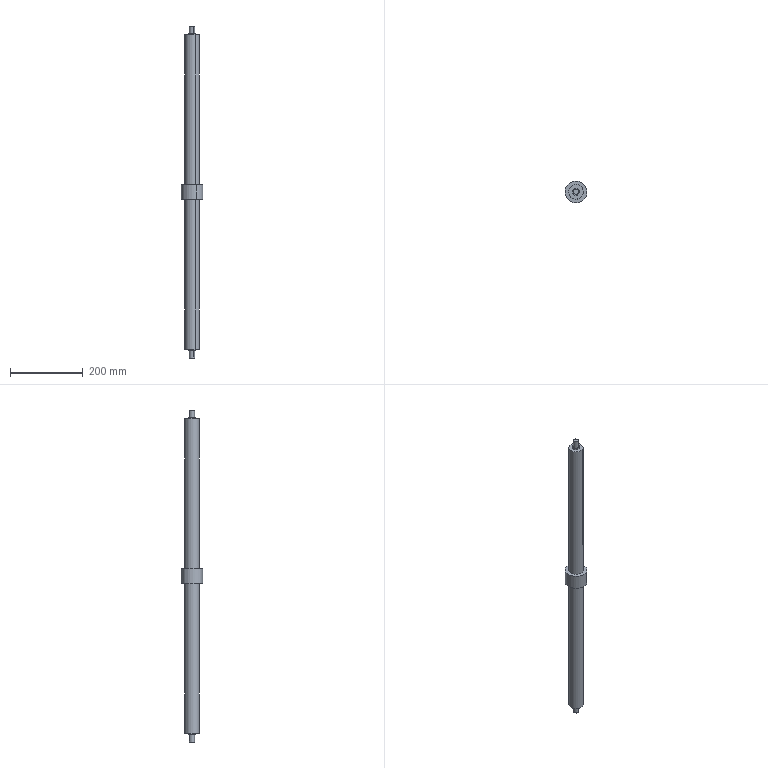Part | SolidWorks | features BaseBody 1 | 1 solid | 34 faces | box 60 x 60 x 912 mm | volume 1156729 mm3 | plane 24 | cylinder 10 | commonest cylinder face diameters 14 x4 40 x4 60 x2
STEP:
#1=CARTESIAN_POINT('',(-440.034,50.813,456.));
#2=VERTEX_POINT('',#1);
#3=CARTESIAN_POINT('',(-446.031,63.464,456.));
#4=VERTEX_POINT('',#3);
#5=CARTESIAN_POINT('',(-443.032,57.138,456.));
#6=DIRECTION('',(0.,0.,1.));
#7=DIRECTION('',(0.4284,-0.9036,0.));
#8=AXIS2_PLACEMENT_3D('',#5,#6,#7);
#9=CIRCLE('',#8,7.);
#10=EDGE_CURVE('',#2,#4,#9,.T.);
#11=ORIENTED_EDGE('',*,*,#10,.F.);
#12=CARTESIAN_POINT('',(-440.034,50.813,435.));
#13=VERTEX_POINT('',#12);
#14=CARTESIAN_POINT('',(-440.034,50.813,456.));
#15=DIRECTION('',(0.,0.,-1.));
#16=VECTOR('',#15,1000.);
#17=LINE('',#14,#16);
#18=EDGE_CURVE('',#2,#13,#17,.T.);
#19=ORIENTED_EDGE('',*,*,#18,.T.);
#20=CARTESIAN_POINT('',(-446.031,63.464,435.));
#21=VERTEX_POINT('',#20);
#22=CARTESIAN_POINT('',(-443.032,57.138,435.));
#23=DIRECTION('',(0.,0.,1.));
#24=DIRECTION('',(0.4284,-0.9036,0.));
#25=AXIS2_PLACEMENT_3D('',#22,#23,#24);
#26=CIRCLE('',#25,7.);
#27=EDGE_CURVE('',#13,#21,#26,.T.);
#28=ORIENTED_EDGE('',*,*,#27,.T.);
#29=CARTESIAN_POINT('',(-446.031,63.464,456.));
#30=DIRECTION('',(0.,0.,-1.));
#31=VECTOR('',#30,1000.);
#32=LINE('',#29,#31);
#33=EDGE_CURVE('',#4,#21,#32,.T.);
#34=ORIENTED_EDGE('',*,*,#33,.F.);
#35=EDGE_LOOP('',(#11,#19,#28,#34));
#36=FACE_OUTER_BOUND('',#35,.T.);
#37=CARTESIAN_POINT('',(-443.032,57.138,456.));
#38=DIRECTION('',(0.,0.,-1.));
#39=DIRECTION('',(-0.4284,0.9036,0.));
#40=AXIS2_PLACEMENT_3D('',#37,#38,#39);
#41=CYLINDRICAL_SURFACE('',#40,7.);
#42=ADVANCED_FACE('',(#36),#41,.T.);
#43=CARTESIAN_POINT('',(-446.031,63.464,-456.));
#44=VERTEX_POINT('',#43);
#45=CARTESIAN_POINT('',(-440.034,50.813,-456.));
#46=VERTEX_POINT('',#45);
#47=CARTESIAN_POINT('',(-443.032,57.138,-456.));
#48=DIRECTION('',(0.,0.,-1.));
#49=DIRECTION('',(-0.4284,0.9036,0.));
#50=AXIS2_PLACEMENT_3D('',#47,#48,#49);
#51=CIRCLE('',#50,7.);
#52=EDGE_CURVE('',#44,#46,#51,.T.);
#53=ORIENTED_EDGE('',*,*,#52,.F.);
#54=CARTESIAN_POINT('',(-446.031,63.464,-435.));
#55=VERTEX_POINT('',#54);
#56=CARTESIAN_POINT('',(-446.031,63.464,-456.));
#57=DIRECTION('',(0.,0.,1.));
#58=VECTOR('',#57,1000.);
#59=LINE('',#56,#58);
#60=EDGE_CURVE('',#44,#55,#59,.T.);
#61=ORIENTED_EDGE('',*,*,#60,.T.);
#62=CARTESIAN_POINT('',(-440.034,50.813,-435.));
#63=VERTEX_POINT('',#62);
#64=CARTESIAN_POINT('',(-443.032,57.138,-435.));
#65=DIRECTION('',(0.,0.,-1.));
#66=DIRECTION('',(-0.4284,0.9036,0.));
#67=AXIS2_PLACEMENT_3D('',#64,#65,#66);
#68=CIRCLE('',#67,7.);
#69=EDGE_CURVE('',#55,#63,#68,.T.);
#70=ORIENTED_EDGE('',*,*,#69,.T.);
#71=CARTESIAN_POINT('',(-440.034,50.813,-456.));
#72=DIRECTION('',(0.,0.,1.));
#73=VECTOR('',#72,1000.);
#74=LINE('',#71,#73);
#75=EDGE_CURVE('',#46,#63,#74,.T.);
#76=ORIENTED_EDGE('',*,*,#75,.F.);
#77=EDGE_LOOP('',(#53,#61,#70,#76));
#78=FACE_OUTER_BOUND('',#77,.T.);
#79=CARTESIAN_POINT('',(-443.032,57.138,-456.));
#80=DIRECTION('',(0.,0.,1.));
#81=DIRECTION('',(0.4284,-0.9036,0.));
#82=AXIS2_PLACEMENT_3D('',#79,#80,#81);
#83=CYLINDRICAL_SURFACE('',#82,7.);
#84=ADVANCED_FACE('',(#78),#83,.T.);
#85=CARTESIAN_POINT('',(-430.181,30.03,20.));
#86=VERTEX_POINT('',#85);
#87=CARTESIAN_POINT('',(-455.884,84.246,20.));
#88=VERTEX_POINT('',#87);
#89=CARTESIAN_POINT('',(-443.032,57.138,20.));
#90=DIRECTION('',(0.,0.,1.));
#91=DIRECTION('',(0.4284,-0.9036,0.));
#92=AXIS2_PLACEMENT_3D('',#89,#90,#91);
#93=CIRCLE('',#92,30.);
#94=EDGE_CURVE('',#86,#88,#93,.T.);
#95=ORIENTED_EDGE('',*,*,#94,.F.);
#96=CARTESIAN_POINT('',(-430.181,30.03,-20.));
#97=VERTEX_POINT('',#96);
#98=CARTESIAN_POINT('',(-430.181,30.03,20.));
#99=DIRECTION('',(0.,0.,-1.));
#100=VECTOR('',#99,1000.);
#101=LINE('',#98,#100);
#102=EDGE_CURVE('',#86,#97,#101,.T.);
#103=ORIENTED_EDGE('',*,*,#102,.T.);
#104=CARTESIAN_POINT('',(-455.884,84.246,-20.));
#105=VERTEX_POINT('',#104);
#106=CARTESIAN_POINT('',(-443.032,57.138,-20.));
#107=DIRECTION('',(0.,0.,1.));
#108=DIRECTION('',(0.4284,-0.9036,0.));
#109=AXIS2_PLACEMENT_3D('',#106,#107,#108);
#110=CIRCLE('',#109,30.);
#111=EDGE_CURVE('',#97,#105,#110,.T.);
#112=ORIENTED_EDGE('',*,*,#111,.T.);
#113=CARTESIAN_POINT('',(-455.884,84.246,20.));
#114=DIRECTION('',(0.,0.,-1.));
#115=VECTOR('',#114,1000.);
#116=LINE('',#113,#115);
#117=EDGE_CURVE('',#88,#105,#116,.T.);
#118=ORIENTED_EDGE('',*,*,#117,.F.);
#119=EDGE_LOOP('',(#95,#103,#112,#118));
#120=FACE_OUTER_BOUND('',#119,.T.);
#121=CARTESIAN_POINT('',(-443.032,57.138,20.));
#122=DIRECTION('',(0.,0.,-1.));
#123=DIRECTION('',(-0.4284,0.9036,0.));
#124=AXIS2_PLACEMENT_3D('',#121,#122,#123);
#125=CYLINDRICAL_SURFACE('',#124,30.);
#126=ADVANCED_FACE('',(#120),#125,.T.);
#127=CARTESIAN_POINT('',(-434.465,39.066,-20.));
#128=VERTEX_POINT('',#127);
#129=CARTESIAN_POINT('',(-451.6,75.21,-20.));
#130=VERTEX_POINT('',#129);
#131=CARTESIAN_POINT('',(-443.032,57.138,-20.));
#132=DIRECTION('',(0.,0.,1.));
#133=DIRECTION('',(0.4284,-0.9036,0.));
#134=AXIS2_PLACEMENT_3D('',#131,#132,#133);
#135=CIRCLE('',#134,20.);
#136=EDGE_CURVE('',#128,#130,#135,.T.);
#137=ORIENTED_EDGE('',*,*,#136,.F.);
#138=CARTESIAN_POINT('',(-434.465,39.066,-432.));
#139=VERTEX_POINT('',#138);
#140=CARTESIAN_POINT('',(-434.465,39.066,445.));
#141=DIRECTION('',(0.,0.,-1.));
#142=VECTOR('',#141,1000.);
#143=LINE('',#140,#142);
#144=EDGE_CURVE('',#128,#139,#143,.T.);
#145=ORIENTED_EDGE('',*,*,#144,.T.);
#146=CARTESIAN_POINT('',(-451.6,75.21,-432.));
#147=VERTEX_POINT('',#146);
#148=CARTESIAN_POINT('',(-443.032,57.138,-432.));
#149=DIRECTION('',(0.,0.,-1.));
#150=DIRECTION('',(-0.4284,0.9036,0.));
#151=AXIS2_PLACEMENT_3D('',#148,#149,#150);
#152=CIRCLE('',#151,20.);
#153=EDGE_CURVE('',#147,#139,#152,.T.);
#154=ORIENTED_EDGE('',*,*,#153,.F.);
#155=CARTESIAN_POINT('',(-451.6,75.21,445.));
#156=DIRECTION('',(0.,0.,-1.));
#157=VECTOR('',#156,1000.);
#158=LINE('',#155,#157);
#159=EDGE_CURVE('',#130,#147,#158,.T.);
#160=ORIENTED_EDGE('',*,*,#159,.F.);
#161=EDGE_LOOP('',(#137,#145,#154,#160));
#162=FACE_OUTER_BOUND('',#161,.T.);
#163=CARTESIAN_POINT('',(-443.032,57.138,445.));
#164=DIRECTION('',(0.,0.,-1.));
#165=DIRECTION('',(-0.4284,0.9036,0.));
#166=AXIS2_PLACEMENT_3D('',#163,#164,#165);
#167=CYLINDRICAL_SURFACE('',#166,20.);
#168=ADVANCED_FACE('',(#162),#167,.T.);
#169=CARTESIAN_POINT('',(-434.465,39.066,432.));
#170=VERTEX_POINT('',#169);
#171=CARTESIAN_POINT('',(-451.6,75.21,432.));
#172=VERTEX_POINT('',#171);
#173=CARTESIAN_POINT('',(-443.032,57.138,432.));
#174=DIRECTION('',(0.,0.,1.));
#175=DIRECTION('',(0.4284,-0.9036,0.));
#176=AXIS2_PLACEMENT_3D('',#173,#174,#175);
#177=CIRCLE('',#176,20.);
#178=EDGE_CURVE('',#170,#172,#177,.T.);
#179=ORIENTED_EDGE('',*,*,#178,.F.);
#180=CARTESIAN_POINT('',(-434.465,39.066,20.));
#181=VERTEX_POINT('',#180);
#182=CARTESIAN_POINT('',(-434.465,39.066,445.));
#183=DIRECTION('',(0.,0.,-1.));
#184=VECTOR('',#183,1000.);
#185=LINE('',#182,#184);
#186=EDGE_CURVE('',#170,#181,#185,.T.);
#187=ORIENTED_EDGE('',*,*,#186,.T.);
#188=CARTESIAN_POINT('',(-451.6,75.21,20.));
#189=VERTEX_POINT('',#188);
#190=CARTESIAN_POINT('',(-443.032,57.138,20.));
#191=DIRECTION('',(0.,0.,1.));
#192=DIRECTION('',(0.4284,-0.9036,0.));
#193=AXIS2_PLACEMENT_3D('',#190,#191,#192);
#194=CIRCLE('',#193,20.);
#195=EDGE_CURVE('',#181,#189,#194,.T.);
#196=ORIENTED_EDGE('',*,*,#195,.T.);
#197=CARTESIAN_POINT('',(-451.6,75.21,445.));
#198=DIRECTION('',(0.,0.,-1.));
#199=VECTOR('',#198,1000.);
#200=LINE('',#197,#199);
#201=EDGE_CURVE('',#172,#189,#200,.T.);
#202=ORIENTED_EDGE('',*,*,#201,.F.);
#203=EDGE_LOOP('',(#179,#187,#196,#202));
#204=FACE_OUTER_BOUND('',#203,.T.);
#205=CARTESIAN_POINT('',(-443.032,57.138,445.));
#206=DIRECTION('',(0.,0.,-1.));
#207=DIRECTION('',(-0.4284,0.9036,0.));
#208=AXIS2_PLACEMENT_3D('',#205,#206,#207);
#209=CYLINDRICAL_SURFACE('',#208,20.);
#210=ADVANCED_FACE('',(#204),#209,.T.);
#211=ORIENTED_EDGE('',*,*,#186,.F.);
#212=CARTESIAN_POINT('',(-443.032,57.138,432.));
#213=DIRECTION('',(0.,0.,1.));
#214=DIRECTION('',(0.4284,-0.9036,0.));
#215=AXIS2_PLACEMENT_3D('',#212,#213,#214);
#216=CIRCLE('',#215,20.);
#217=EDGE_CURVE('',#172,#170,#216,.T.);
#218=ORIENTED_EDGE('',*,*,#217,.F.);
#219=ORIENTED_EDGE('',*,*,#201,.T.);
#220=CARTESIAN_POINT('',(-443.032,57.138,20.));
#221=DIRECTION('',(0.,0.,1.));
#222=DIRECTION('',(0.4284,-0.9036,0.));
#223=AXIS2_PLACEMENT_3D('',#220,#221,#222);
#224=CIRCLE('',#223,20.);
#225=EDGE_CURVE('',#189,#181,#224,.T.);
#226=ORIENTED_EDGE('',*,*,#225,.T.);
#227=EDGE_LOOP('',(#211,#218,#219,#226));
#228=FACE_OUTER_BOUND('',#227,.T.);
#229=CARTESIAN_POINT('',(-443.032,57.138,445.));
#230=DIRECTION('',(0.,0.,-1.));
#231=DIRECTION('',(-0.4284,0.9036,0.));
#232=AXIS2_PLACEMENT_3D('',#229,#230,#231);
#233=CYLINDRICAL_SURFACE('',#232,20.);
#234=ADVANCED_FACE('',(#228),#233,.T.);
#235=ORIENTED_EDGE('',*,*,#144,.F.);
#236=CARTESIAN_POINT('',(-443.032,57.138,-20.));
#237=DIRECTION('',(0.,0.,1.));
#238=DIRECTION('',(0.4284,-0.9036,0.));
#239=AXIS2_PLACEMENT_3D('',#236,#237,#238);
#240=CIRCLE('',#239,20.);
#241=EDGE_CURVE('',#130,#128,#240,.T.);
#242=ORIENTED_EDGE('',*,*,#241,.F.);
#243=ORIENTED_EDGE('',*,*,#159,.T.);
#244=CARTESIAN_POINT('',(-443.032,57.138,-432.));
#245=DIRECTION('',(0.,0.,-1.));
#246=DIRECTION('',(-0.4284,0.9036,0.));
#247=AXIS2_PLACEMENT_3D('',#244,#245,#246);
#248=CIRCLE('',#247,20.);
#249=EDGE_CURVE('',#139,#147,#248,.T.);
#250=ORIENTED_EDGE('',*,*,#249,.F.);
#251=EDGE_LOOP('',(#235,#242,#243,#250));
#252=FACE_OUTER_BOUND('',#251,.T.);
#253=CARTESIAN_POINT('',(-443.032,57.138,445.));
#254=DIRECTION('',(0.,0.,-1.));
#255=DIRECTION('',(-0.4284,0.9036,0.));
#256=AXIS2_PLACEMENT_3D('',#253,#254,#255);
#257=CYLINDRICAL_SURFACE('',#256,20.);
#258=ADVANCED_FACE('',(#252),#257,.T.);
#259=CARTESIAN_POINT('',(-443.032,57.138,20.));
#260=DIRECTION('',(0.,0.,1.));
#261=DIRECTION('',(0.4284,-0.9036,0.));
#262=AXIS2_PLACEMENT_3D('',#259,#260,#261);
#263=CIRCLE('',#262,30.);
#264=EDGE_CURVE('',#88,#86,#263,.T.);
#265=ORIENTED_EDGE('',*,*,#264,.T.);
#266=ORIENTED_EDGE('',*,*,#94,.T.);
#267=EDGE_LOOP('',(#265,#266));
#268=FACE_OUTER_BOUND('',#267,.T.);
#269=ORIENTED_EDGE('',*,*,#225,.F.);
#270=ORIENTED_EDGE('',*,*,#195,.F.);
#271=EDGE_LOOP('',(#269,#270));
#272=FACE_BOUND('',#271,.T.);
#273=CARTESIAN_POINT('',(-443.032,57.138,20.));
#274=DIRECTION('',(0.,0.,1.));
#275=DIRECTION('',(0.4284,-0.9036,0.));
#276=AXIS2_PLACEMENT_3D('',#273,#274,#275);
#277=PLANE('',#276);
#278=ADVANCED_FACE('',(#268,#272),#277,.T.);
#279=CARTESIAN_POINT('',(-443.032,57.138,-20.));
#280=DIRECTION('',(0.,0.,1.));
#281=DIRECTION('',(0.4284,-0.9036,0.));
#282=AXIS2_PLACEMENT_3D('',#279,#280,#281);
#283=CIRCLE('',#282,30.);
#284=EDGE_CURVE('',#105,#97,#283,.T.);
#285=ORIENTED_EDGE('',*,*,#284,.F.);
#286=ORIENTED_EDGE('',*,*,#111,.F.);
#287=EDGE_LOOP('',(#285,#286));
#288=FACE_OUTER_BOUND('',#287,.T.);
#289=ORIENTED_EDGE('',*,*,#241,.T.);
#290=ORIENTED_EDGE('',*,*,#136,.T.);
#291=EDGE_LOOP('',(#289,#290));
#292=FACE_BOUND('',#291,.T.);
#293=CARTESIAN_POINT('',(-443.032,57.138,-20.));
#294=DIRECTION('',(0.,0.,1.));
#295=DIRECTION('',(0.4284,-0.9036,0.));
#296=AXIS2_PLACEMENT_3D('',#293,#294,#295);
#297=PLANE('',#296);
#298=ADVANCED_FACE('',(#288,#292),#297,.F.);
#299=ORIENTED_EDGE('',*,*,#102,.F.);
#300=ORIENTED_EDGE('',*,*,#264,.F.);
#301=ORIENTED_EDGE('',*,*,#117,.T.);
#302=ORIENTED_EDGE('',*,*,#284,.T.);
#303=EDGE_LOOP('',(#299,#300,#301,#302));
#304=FACE_OUTER_BOUND('',#303,.T.);
#305=CARTESIAN_POINT('',(-443.032,57.138,20.));
#306=DIRECTION('',(0.,0.,-1.));
#307=DIRECTION('',(-0.4284,0.9036,0.));
#308=AXIS2_PLACEMENT_3D('',#305,#306,#307);
#309=CYLINDRICAL_SURFACE('',#308,30.);
#310=ADVANCED_FACE('',(#304),#309,.T.);
#311=ORIENTED_EDGE('',*,*,#153,.T.);
#312=ORIENTED_EDGE('',*,*,#249,.T.);
#313=EDGE_LOOP('',(#311,#312));
#314=FACE_OUTER_BOUND('',#313,.T.);
#315=CARTESIAN_POINT('',(-447.316,66.174,-432.));
#316=VERTEX_POINT('',#315);
#317=CARTESIAN_POINT('',(-439.672,66.557,-432.));
#318=VERTEX_POINT('',#317);
#319=CARTESIAN_POINT('',(-439.672,66.557,-432.));
#320=DIRECTION('',(0.9987,0.04998,0.));
#321=VECTOR('',#320,1000.);
#322=LINE('',#319,#321);
#323=EDGE_CURVE('',#316,#318,#322,.T.);
#324=ORIENTED_EDGE('',*,*,#323,.F.);
#325=CARTESIAN_POINT('',(-452.451,60.499,-432.));
#326=VERTEX_POINT('',#325);
#327=CARTESIAN_POINT('',(-452.451,60.499,-432.));
#328=DIRECTION('',(0.6709,0.7416,0.));
#329=VECTOR('',#328,1000.);
#330=LINE('',#327,#329);
#331=EDGE_CURVE('',#326,#316,#330,.T.);
#332=ORIENTED_EDGE('',*,*,#331,.F.);
#333=CARTESIAN_POINT('',(-452.068,52.855,-432.));
#334=VERTEX_POINT('',#333);
#335=CARTESIAN_POINT('',(-452.068,52.855,-432.));
#336=DIRECTION('',(-0.04998,0.9987,0.));
#337=VECTOR('',#336,1000.);
#338=LINE('',#335,#337);
#339=EDGE_CURVE('',#334,#326,#338,.T.);
#340=ORIENTED_EDGE('',*,*,#339,.F.);
#341=CARTESIAN_POINT('',(-446.393,47.72,-432.));
#342=VERTEX_POINT('',#341);
#343=CARTESIAN_POINT('',(-452.068,52.855,-432.));
#344=DIRECTION('',(-0.7416,0.6709,0.));
#345=VECTOR('',#344,1000.);
#346=LINE('',#343,#345);
#347=EDGE_CURVE('',#342,#334,#346,.T.);
#348=ORIENTED_EDGE('',*,*,#347,.F.);
#349=CARTESIAN_POINT('',(-438.748,48.102,-432.));
#350=VERTEX_POINT('',#349);
#351=CARTESIAN_POINT('',(-446.393,47.72,-432.));
#352=DIRECTION('',(-0.9987,-0.04998,0.));
#353=VECTOR('',#352,1000.);
#354=LINE('',#351,#353);
#355=EDGE_CURVE('',#350,#342,#354,.T.);
#356=ORIENTED_EDGE('',*,*,#355,.F.);
#357=CARTESIAN_POINT('',(-433.614,53.778,-432.));
#358=VERTEX_POINT('',#357);
#359=CARTESIAN_POINT('',(-433.614,53.778,-432.));
#360=DIRECTION('',(-0.6709,-0.7416,0.));
#361=VECTOR('',#360,1000.);
#362=LINE('',#359,#361);
#363=EDGE_CURVE('',#358,#350,#362,.T.);
#364=ORIENTED_EDGE('',*,*,#363,.F.);
#365=CARTESIAN_POINT('',(-433.996,61.422,-432.));
#366=VERTEX_POINT('',#365);
#367=CARTESIAN_POINT('',(-433.996,61.422,-432.));
#368=DIRECTION('',(0.04998,-0.9987,0.));
#369=VECTOR('',#368,1000.);
#370=LINE('',#367,#369);
#371=EDGE_CURVE('',#366,#358,#370,.T.);
#372=ORIENTED_EDGE('',*,*,#371,.F.);
#373=CARTESIAN_POINT('',(-433.996,61.422,-432.));
#374=DIRECTION('',(0.7416,-0.6709,0.));
#375=VECTOR('',#374,1000.);
#376=LINE('',#373,#375);
#377=EDGE_CURVE('',#318,#366,#376,.T.);
#378=ORIENTED_EDGE('',*,*,#377,.F.);
#379=EDGE_LOOP('',(#324,#332,#340,#348,#356,#364,#372,#378));
#380=FACE_BOUND('',#379,.T.);
#381=CARTESIAN_POINT('',(-443.032,57.138,-432.));
#382=DIRECTION('',(0.,0.,-1.));
#383=DIRECTION('',(-0.4284,0.9036,0.));
#384=AXIS2_PLACEMENT_3D('',#381,#382,#383);
#385=PLANE('',#384);
#386=ADVANCED_FACE('',(#314,#380),#385,.T.);
#387=CARTESIAN_POINT('',(-439.672,66.557,-435.));
#388=VERTEX_POINT('',#387);
#389=CARTESIAN_POINT('',(-433.996,61.422,-435.));
#390=VERTEX_POINT('',#389);
#391=CARTESIAN_POINT('',(-433.996,61.422,-435.));
#392=DIRECTION('',(0.7416,-0.6709,0.));
#393=VECTOR('',#392,1000.);
#394=LINE('',#391,#393);
#395=EDGE_CURVE('',#388,#390,#394,.T.);
#396=ORIENTED_EDGE('',*,*,#395,.F.);
#397=CARTESIAN_POINT('',(-439.672,66.557,-432.));
#398=DIRECTION('',(0.,0.,-1.));
#399=VECTOR('',#398,1000.);
#400=LINE('',#397,#399);
#401=EDGE_CURVE('',#318,#388,#400,.T.);
#402=ORIENTED_EDGE('',*,*,#401,.F.);
#403=ORIENTED_EDGE('',*,*,#377,.T.);
#404=CARTESIAN_POINT('',(-433.996,61.422,-432.));
#405=DIRECTION('',(0.,0.,-1.));
#406=VECTOR('',#405,1000.);
#407=LINE('',#404,#406);
#408=EDGE_CURVE('',#366,#390,#407,.T.);
#409=ORIENTED_EDGE('',*,*,#408,.T.);
#410=EDGE_LOOP('',(#396,#402,#403,#409));
#411=FACE_OUTER_BOUND('',#410,.T.);
#412=CARTESIAN_POINT('',(-433.996,61.422,-432.));
#413=DIRECTION('',(0.6709,0.7416,0.));
#414=DIRECTION('',(-0.7416,0.6709,0.));
#415=AXIS2_PLACEMENT_3D('',#412,#413,#414);
#416=PLANE('',#415);
#417=ADVANCED_FACE('',(#411),#416,.T.);
#418=CARTESIAN_POINT('',(-447.316,66.174,-435.));
#419=VERTEX_POINT('',#418);
#420=CARTESIAN_POINT('',(-439.672,66.557,-435.));
#421=DIRECTION('',(0.9987,0.04998,0.));
#422=VECTOR('',#421,1000.);
#423=LINE('',#420,#422);
#424=EDGE_CURVE('',#419,#388,#423,.T.);
#425=ORIENTED_EDGE('',*,*,#424,.F.);
#426=CARTESIAN_POINT('',(-447.316,66.174,-432.));
#427=DIRECTION('',(0.,0.,-1.));
#428=VECTOR('',#427,1000.);
#429=LINE('',#426,#428);
#430=EDGE_CURVE('',#316,#419,#429,.T.);
#431=ORIENTED_EDGE('',*,*,#430,.F.);
#432=ORIENTED_EDGE('',*,*,#323,.T.);
#433=ORIENTED_EDGE('',*,*,#401,.T.);
#434=EDGE_LOOP('',(#425,#431,#432,#433));
#435=FACE_OUTER_BOUND('',#434,.T.);
#436=CARTESIAN_POINT('',(-439.672,66.557,-432.));
#437=DIRECTION('',(-0.04998,0.9987,0.));
#438=DIRECTION('',(-0.9987,-0.04998,0.));
#439=AXIS2_PLACEMENT_3D('',#436,#437,#438);
#440=PLANE('',#439);
#441=ADVANCED_FACE('',(#435),#440,.T.);
#442=CARTESIAN_POINT('',(-452.451,60.499,-435.));
#443=VERTEX_POINT('',#442);
#444=CARTESIAN_POINT('',(-452.451,60.499,-435.));
#445=DIRECTION('',(0.6709,0.7416,0.));
#446=VECTOR('',#445,1000.);
#447=LINE('',#444,#446);
#448=EDGE_CURVE('',#443,#419,#447,.T.);
#449=ORIENTED_EDGE('',*,*,#448,.F.);
#450=CARTESIAN_POINT('',(-452.451,60.499,-432.));
#451=DIRECTION('',(0.,0.,-1.));
#452=VECTOR('',#451,1000.);
#453=LINE('',#450,#452);
#454=EDGE_CURVE('',#326,#443,#453,.T.);
#455=ORIENTED_EDGE('',*,*,#454,.F.);
#456=ORIENTED_EDGE('',*,*,#331,.T.);
#457=ORIENTED_EDGE('',*,*,#430,.T.);
#458=EDGE_LOOP('',(#449,#455,#456,#457));
#459=FACE_OUTER_BOUND('',#458,.T.);
#460=CARTESIAN_POINT('',(-452.451,60.499,-432.));
#461=DIRECTION('',(-0.7416,0.6709,0.));
#462=DIRECTION('',(-0.6709,-0.7416,0.));
#463=AXIS2_PLACEMENT_3D('',#460,#461,#462);
#464=PLANE('',#463);
#465=ADVANCED_FACE('',(#459),#464,.T.);
#466=CARTESIAN_POINT('',(-452.068,52.855,-435.));
#467=VERTEX_POINT('',#466);
#468=CARTESIAN_POINT('',(-452.068,52.855,-435.));
#469=DIRECTION('',(-0.04998,0.9987,0.));
#470=VECTOR('',#469,1000.);
#471=LINE('',#468,#470);
#472=EDGE_CURVE('',#467,#443,#471,.T.);
#473=ORIENTED_EDGE('',*,*,#472,.F.);
#474=CARTESIAN_POINT('',(-452.068,52.855,-432.));
#475=DIRECTION('',(0.,0.,-1.));
#476=VECTOR('',#475,1000.);
#477=LINE('',#474,#476);
#478=EDGE_CURVE('',#334,#467,#477,.T.);
#479=ORIENTED_EDGE('',*,*,#478,.F.);
#480=ORIENTED_EDGE('',*,*,#339,.T.);
#481=ORIENTED_EDGE('',*,*,#454,.T.);
#482=EDGE_LOOP('',(#473,#479,#480,#481));
#483=FACE_OUTER_BOUND('',#482,.T.);
#484=CARTESIAN_POINT('',(-452.068,52.855,-432.));
#485=DIRECTION('',(-0.9987,-0.04998,0.));
#486=DIRECTION('',(0.04998,-0.9987,0.));
#487=AXIS2_PLACEMENT_3D('',#484,#485,#486);
#488=PLANE('',#487);
#489=ADVANCED_FACE('',(#483),#488,.T.);
#490=CARTESIAN_POINT('',(-446.393,47.72,-435.));
#491=VERTEX_POINT('',#490);
#492=CARTESIAN_POINT('',(-452.068,52.855,-435.));
#493=DIRECTION('',(-0.7416,0.6709,0.));
#494=VECTOR('',#493,1000.);
#495=LINE('',#492,#494);
#496=EDGE_CURVE('',#491,#467,#495,.T.);
#497=ORIENTED_EDGE('',*,*,#496,.F.);
#498=CARTESIAN_POINT('',(-446.393,47.72,-432.));
#499=DIRECTION('',(0.,0.,-1.));
#500=VECTOR('',#499,1000.);
#501=LINE('',#498,#500);
#502=EDGE_CURVE('',#342,#491,#501,.T.);
#503=ORIENTED_EDGE('',*,*,#502,.F.);
#504=ORIENTED_EDGE('',*,*,#347,.T.);
#505=ORIENTED_EDGE('',*,*,#478,.T.);
#506=EDGE_LOOP('',(#497,#503,#504,#505));
#507=FACE_OUTER_BOUND('',#506,.T.);
#508=CARTESIAN_POINT('',(-452.068,52.855,-432.));
#509=DIRECTION('',(-0.6709,-0.7416,0.));
#510=DIRECTION('',(0.7416,-0.6709,0.));
#511=AXIS2_PLACEMENT_3D('',#508,#509,#510);
#512=PLANE('',#511);
#513=ADVANCED_FACE('',(#507),#512,.T.);
#514=CARTESIAN_POINT('',(-438.748,48.102,-435.));
#515=VERTEX_POINT('',#514);
#516=CARTESIAN_POINT('',(-446.393,47.72,-435.));
#517=DIRECTION('',(-0.9987,-0.04998,0.));
#518=VECTOR('',#517,1000.);
#519=LINE('',#516,#518);
#520=EDGE_CURVE('',#515,#491,#519,.T.);
#521=ORIENTED_EDGE('',*,*,#520,.F.);
#522=CARTESIAN_POINT('',(-438.748,48.102,-432.));
#523=DIRECTION('',(0.,0.,-1.));
#524=VECTOR('',#523,1000.);
#525=LINE('',#522,#524);
#526=EDGE_CURVE('',#350,#515,#525,.T.);
#527=ORIENTED_EDGE('',*,*,#526,.F.);
#528=ORIENTED_EDGE('',*,*,#355,.T.);
#529=ORIENTED_EDGE('',*,*,#502,.T.);
#530=EDGE_LOOP('',(#521,#527,#528,#529));
#531=FACE_OUTER_BOUND('',#530,.T.);
#532=CARTESIAN_POINT('',(-446.393,47.72,-432.));
#533=DIRECTION('',(0.04998,-0.9987,0.));
#534=DIRECTION('',(0.9987,0.04998,0.));
#535=AXIS2_PLACEMENT_3D('',#532,#533,#534);
#536=PLANE('',#535);
#537=ADVANCED_FACE('',(#531),#536,.T.);
#538=CARTESIAN_POINT('',(-433.614,53.778,-435.));
#539=VERTEX_POINT('',#538);
#540=CARTESIAN_POINT('',(-433.614,53.778,-435.));
#541=DIRECTION('',(-0.6709,-0.7416,0.));
#542=VECTOR('',#541,1000.);
#543=LINE('',#540,#542);
#544=EDGE_CURVE('',#539,#515,#543,.T.);
#545=ORIENTED_EDGE('',*,*,#544,.F.);
#546=CARTESIAN_POINT('',(-433.614,53.778,-432.));
#547=DIRECTION('',(0.,0.,-1.));
#548=VECTOR('',#547,1000.);
#549=LINE('',#546,#548);
#550=EDGE_CURVE('',#358,#539,#549,.T.);
#551=ORIENTED_EDGE('',*,*,#550,.F.);
#552=ORIENTED_EDGE('',*,*,#363,.T.);
#553=ORIENTED_EDGE('',*,*,#526,.T.);
#554=EDGE_LOOP('',(#545,#551,#552,#553));
#555=FACE_OUTER_BOUND('',#554,.T.);
#556=CARTESIAN_POINT('',(-433.614,53.778,-432.));
#557=DIRECTION('',(0.7416,-0.6709,0.));
#558=DIRECTION('',(0.6709,0.7416,0.));
#559=AXIS2_PLACEMENT_3D('',#556,#557,#558);
#560=PLANE('',#559);
#561=ADVANCED_FACE('',(#555),#560,.T.);
#562=CARTESIAN_POINT('',(-433.996,61.422,-435.));
#563=DIRECTION('',(0.04998,-0.9987,0.));
#564=VECTOR('',#563,1000.);
#565=LINE('',#562,#564);
#566=EDGE_CURVE('',#390,#539,#565,.T.);
#567=ORIENTED_EDGE('',*,*,#566,.F.);
#568=ORIENTED_EDGE('',*,*,#408,.F.);
#569=ORIENTED_EDGE('',*,*,#371,.T.);
#570=ORIENTED_EDGE('',*,*,#550,.T.);
#571=EDGE_LOOP('',(#567,#568,#569,#570));
#572=FACE_OUTER_BOUND('',#571,.T.);
#573=CARTESIAN_POINT('',(-433.996,61.422,-432.));
#574=DIRECTION('',(0.9987,0.04998,0.));
#575=DIRECTION('',(-0.04998,0.9987,0.));
#576=AXIS2_PLACEMENT_3D('',#573,#574,#575);
#577=PLANE('',#576);
#578=ADVANCED_FACE('',(#572),#577,.T.);
#579=CARTESIAN_POINT('',(-443.032,57.138,-456.));
#580=DIRECTION('',(0.,0.,-1.));
#581=DIRECTION('',(-0.4284,0.9036,0.));
#582=AXIS2_PLACEMENT_3D('',#579,#580,#581);
#583=CIRCLE('',#582,7.);
#584=EDGE_CURVE('',#46,#44,#583,.T.);
#585=ORIENTED_EDGE('',*,*,#584,.T.);
#586=ORIENTED_EDGE('',*,*,#52,.T.);
#587=EDGE_LOOP('',(#585,#586));
#588=FACE_OUTER_BOUND('',#587,.T.);
#589=CARTESIAN_POINT('',(-443.032,57.138,-456.));
#590=DIRECTION('',(0.,0.,-1.));
#591=DIRECTION('',(-0.4284,0.9036,0.));
#592=AXIS2_PLACEMENT_3D('',#589,#590,#591);
#593=PLANE('',#592);
#594=ADVANCED_FACE('',(#588),#593,.T.);
#595=ORIENTED_EDGE('',*,*,#60,.F.);
#596=ORIENTED_EDGE('',*,*,#584,.F.);
#597=ORIENTED_EDGE('',*,*,#75,.T.);
#598=CARTESIAN_POINT('',(-443.032,57.138,-435.));
#599=DIRECTION('',(0.,0.,-1.));
#600=DIRECTION('',(-0.4284,0.9036,0.));
#601=AXIS2_PLACEMENT_3D('',#598,#599,#600);
#602=CIRCLE('',#601,7.);
#603=EDGE_CURVE('',#63,#55,#602,.T.);
#604=ORIENTED_EDGE('',*,*,#603,.T.);
#605=EDGE_LOOP('',(#595,#596,#597,#604));
#606=FACE_OUTER_BOUND('',#605,.T.);
#607=CARTESIAN_POINT('',(-443.032,57.138,-456.));
#608=DIRECTION('',(0.,0.,1.));
#609=DIRECTION('',(0.4284,-0.9036,0.));
#610=AXIS2_PLACEMENT_3D('',#607,#608,#609);
#611=CYLINDRICAL_SURFACE('',#610,7.);
#612=ADVANCED_FACE('',(#606),#611,.T.);
#613=ORIENTED_EDGE('',*,*,#603,.F.);
#614=ORIENTED_EDGE('',*,*,#69,.F.);
#615=EDGE_LOOP('',(#613,#614));
#616=FACE_BOUND('',#615,.T.);
#617=ORIENTED_EDGE('',*,*,#424,.T.);
#618=ORIENTED_EDGE('',*,*,#395,.T.);
#619=ORIENTED_EDGE('',*,*,#566,.T.);
#620=ORIENTED_EDGE('',*,*,#544,.T.);
#621=ORIENTED_EDGE('',*,*,#520,.T.);
#622=ORIENTED_EDGE('',*,*,#496,.T.);
#623=ORIENTED_EDGE('',*,*,#472,.T.);
#624=ORIENTED_EDGE('',*,*,#448,.T.);
#625=EDGE_LOOP('',(#617,#618,#619,#620,#621,#622,#623,#624));
#626=FACE_OUTER_BOUND('',#625,.T.);
#627=CARTESIAN_POINT('',(-443.032,57.138,-435.));
#628=DIRECTION('',(0.,0.,-1.));
#629=DIRECTION('',(-0.4284,0.9036,0.));
#630=AXIS2_PLACEMENT_3D('',#627,#628,#629);
#631=PLANE('',#630);
#632=ADVANCED_FACE('',(#616,#626),#631,.T.);
#633=ORIENTED_EDGE('',*,*,#217,.T.);
#634=ORIENTED_EDGE('',*,*,#178,.T.);
#635=EDGE_LOOP('',(#633,#634));
#636=FACE_OUTER_BOUND('',#635,.T.);
#637=CARTESIAN_POINT('',(-433.614,53.778,432.));
#638=VERTEX_POINT('',#637);
#639=CARTESIAN_POINT('',(-433.996,61.422,432.));
#640=VERTEX_POINT('',#639);
#641=CARTESIAN_POINT('',(-433.996,61.422,432.));
#642=DIRECTION('',(-0.04998,0.9987,0.));
#643=VECTOR('',#642,1000.);
#644=LINE('',#641,#643);
#645=EDGE_CURVE('',#638,#640,#644,.T.);
#646=ORIENTED_EDGE('',*,*,#645,.F.);
#647=CARTESIAN_POINT('',(-438.748,48.102,432.));
#648=VERTEX_POINT('',#647);
#649=CARTESIAN_POINT('',(-433.614,53.778,432.));
#650=DIRECTION('',(0.6709,0.7416,0.));
#651=VECTOR('',#650,1000.);
#652=LINE('',#649,#651);
#653=EDGE_CURVE('',#648,#638,#652,.T.);
#654=ORIENTED_EDGE('',*,*,#653,.F.);
#655=CARTESIAN_POINT('',(-446.393,47.72,432.));
#656=VERTEX_POINT('',#655);
#657=CARTESIAN_POINT('',(-446.393,47.72,432.));
#658=DIRECTION('',(0.9987,0.04998,0.));
#659=VECTOR('',#658,1000.);
#660=LINE('',#657,#659);
#661=EDGE_CURVE('',#656,#648,#660,.T.);
#662=ORIENTED_EDGE('',*,*,#661,.F.);
#663=CARTESIAN_POINT('',(-452.068,52.855,432.));
#664=VERTEX_POINT('',#663);
#665=CARTESIAN_POINT('',(-452.068,52.855,432.));
#666=DIRECTION('',(0.7416,-0.6709,0.));
#667=VECTOR('',#666,1000.);
#668=LINE('',#665,#667);
#669=EDGE_CURVE('',#664,#656,#668,.T.);
#670=ORIENTED_EDGE('',*,*,#669,.F.);
#671=CARTESIAN_POINT('',(-452.451,60.499,432.));
#672=VERTEX_POINT('',#671);
#673=CARTESIAN_POINT('',(-452.068,52.855,432.));
#674=DIRECTION('',(0.04998,-0.9987,0.));
#675=VECTOR('',#674,1000.);
#676=LINE('',#673,#675);
#677=EDGE_CURVE('',#672,#664,#676,.T.);
#678=ORIENTED_EDGE('',*,*,#677,.F.);
#679=CARTESIAN_POINT('',(-447.316,66.174,432.));
#680=VERTEX_POINT('',#679);
#681=CARTESIAN_POINT('',(-452.451,60.499,432.));
#682=DIRECTION('',(-0.6709,-0.7416,0.));
#683=VECTOR('',#682,1000.);
#684=LINE('',#681,#683);
#685=EDGE_CURVE('',#680,#672,#684,.T.);
#686=ORIENTED_EDGE('',*,*,#685,.F.);
#687=CARTESIAN_POINT('',(-439.672,66.557,432.));
#688=VERTEX_POINT('',#687);
#689=CARTESIAN_POINT('',(-439.672,66.557,432.));
#690=DIRECTION('',(-0.9987,-0.04998,0.));
#691=VECTOR('',#690,1000.);
#692=LINE('',#689,#691);
#693=EDGE_CURVE('',#688,#680,#692,.T.);
#694=ORIENTED_EDGE('',*,*,#693,.F.);
#695=CARTESIAN_POINT('',(-433.996,61.422,432.));
#696=DIRECTION('',(-0.7416,0.6709,0.));
#697=VECTOR('',#696,1000.);
#698=LINE('',#695,#697);
#699=EDGE_CURVE('',#640,#688,#698,.T.);
#700=ORIENTED_EDGE('',*,*,#699,.F.);
#701=EDGE_LOOP('',(#646,#654,#662,#670,#678,#686,#694,#700));
#702=FACE_BOUND('',#701,.T.);
#703=CARTESIAN_POINT('',(-443.032,57.138,432.));
#704=DIRECTION('',(0.,0.,1.));
#705=DIRECTION('',(0.4284,-0.9036,0.));
#706=AXIS2_PLACEMENT_3D('',#703,#704,#705);
#707=PLANE('',#706);
#708=ADVANCED_FACE('',(#636,#702),#707,.T.);
#709=CARTESIAN_POINT('',(-433.614,53.778,435.));
#710=VERTEX_POINT('',#709);
#711=CARTESIAN_POINT('',(-433.996,61.422,435.));
#712=VERTEX_POINT('',#711);
#713=CARTESIAN_POINT('',(-433.996,61.422,435.));
#714=DIRECTION('',(-0.04998,0.9987,0.));
#715=VECTOR('',#714,1000.);
#716=LINE('',#713,#715);
#717=EDGE_CURVE('',#710,#712,#716,.T.);
#718=ORIENTED_EDGE('',*,*,#717,.F.);
#719=CARTESIAN_POINT('',(-433.614,53.778,432.));
#720=DIRECTION('',(0.,0.,1.));
#721=VECTOR('',#720,1000.);
#722=LINE('',#719,#721);
#723=EDGE_CURVE('',#638,#710,#722,.T.);
#724=ORIENTED_EDGE('',*,*,#723,.F.);
#725=ORIENTED_EDGE('',*,*,#645,.T.);
#726=CARTESIAN_POINT('',(-433.996,61.422,432.));
#727=DIRECTION('',(0.,0.,1.));
#728=VECTOR('',#727,1000.);
#729=LINE('',#726,#728);
#730=EDGE_CURVE('',#640,#712,#729,.T.);
#731=ORIENTED_EDGE('',*,*,#730,.T.);
#732=EDGE_LOOP('',(#718,#724,#725,#731));
#733=FACE_OUTER_BOUND('',#732,.T.);
#734=CARTESIAN_POINT('',(-433.996,61.422,432.));
#735=DIRECTION('',(0.9987,0.04998,0.));
#736=DIRECTION('',(-0.04998,0.9987,0.));
#737=AXIS2_PLACEMENT_3D('',#734,#735,#736);
#738=PLANE('',#737);
#739=ADVANCED_FACE('',(#733),#738,.T.);
#740=CARTESIAN_POINT('',(-438.748,48.102,435.));
#741=VERTEX_POINT('',#740);
#742=CARTESIAN_POINT('',(-433.614,53.778,435.));
#743=DIRECTION('',(0.6709,0.7416,0.));
#744=VECTOR('',#743,1000.);
#745=LINE('',#742,#744);
#746=EDGE_CURVE('',#741,#710,#745,.T.);
#747=ORIENTED_EDGE('',*,*,#746,.F.);
#748=CARTESIAN_POINT('',(-438.748,48.102,432.));
#749=DIRECTION('',(0.,0.,1.));
#750=VECTOR('',#749,1000.);
#751=LINE('',#748,#750);
#752=EDGE_CURVE('',#648,#741,#751,.T.);
#753=ORIENTED_EDGE('',*,*,#752,.F.);
#754=ORIENTED_EDGE('',*,*,#653,.T.);
#755=ORIENTED_EDGE('',*,*,#723,.T.);
#756=EDGE_LOOP('',(#747,#753,#754,#755));
#757=FACE_OUTER_BOUND('',#756,.T.);
#758=CARTESIAN_POINT('',(-433.614,53.778,432.));
#759=DIRECTION('',(0.7416,-0.6709,0.));
#760=DIRECTION('',(0.6709,0.7416,0.));
#761=AXIS2_PLACEMENT_3D('',#758,#759,#760);
#762=PLANE('',#761);
#763=ADVANCED_FACE('',(#757),#762,.T.);
#764=CARTESIAN_POINT('',(-446.393,47.72,435.));
#765=VERTEX_POINT('',#764);
#766=CARTESIAN_POINT('',(-446.393,47.72,435.));
#767=DIRECTION('',(0.9987,0.04998,0.));
#768=VECTOR('',#767,1000.);
#769=LINE('',#766,#768);
#770=EDGE_CURVE('',#765,#741,#769,.T.);
#771=ORIENTED_EDGE('',*,*,#770,.F.);
#772=CARTESIAN_POINT('',(-446.393,47.72,432.));
#773=DIRECTION('',(0.,0.,1.));
#774=VECTOR('',#773,1000.);
#775=LINE('',#772,#774);
#776=EDGE_CURVE('',#656,#765,#775,.T.);
#777=ORIENTED_EDGE('',*,*,#776,.F.);
#778=ORIENTED_EDGE('',*,*,#661,.T.);
#779=ORIENTED_EDGE('',*,*,#752,.T.);
#780=EDGE_LOOP('',(#771,#777,#778,#779));
#781=FACE_OUTER_BOUND('',#780,.T.);
#782=CARTESIAN_POINT('',(-446.393,47.72,432.));
#783=DIRECTION('',(0.04998,-0.9987,0.));
#784=DIRECTION('',(0.9987,0.04998,0.));
#785=AXIS2_PLACEMENT_3D('',#782,#783,#784);
#786=PLANE('',#785);
#787=ADVANCED_FACE('',(#781),#786,.T.);
#788=CARTESIAN_POINT('',(-452.068,52.855,435.));
#789=VERTEX_POINT('',#788);
#790=CARTESIAN_POINT('',(-452.068,52.855,435.));
#791=DIRECTION('',(0.7416,-0.6709,0.));
#792=VECTOR('',#791,1000.);
#793=LINE('',#790,#792);
#794=EDGE_CURVE('',#789,#765,#793,.T.);
#795=ORIENTED_EDGE('',*,*,#794,.F.);
#796=CARTESIAN_POINT('',(-452.068,52.855,432.));
#797=DIRECTION('',(0.,0.,1.));
#798=VECTOR('',#797,1000.);
#799=LINE('',#796,#798);
#800=EDGE_CURVE('',#664,#789,#799,.T.);
#801=ORIENTED_EDGE('',*,*,#800,.F.);
#802=ORIENTED_EDGE('',*,*,#669,.T.);
#803=ORIENTED_EDGE('',*,*,#776,.T.);
#804=EDGE_LOOP('',(#795,#801,#802,#803));
#805=FACE_OUTER_BOUND('',#804,.T.);
#806=CARTESIAN_POINT('',(-452.068,52.855,432.));
#807=DIRECTION('',(-0.6709,-0.7416,0.));
#808=DIRECTION('',(0.7416,-0.6709,0.));
#809=AXIS2_PLACEMENT_3D('',#806,#807,#808);
#810=PLANE('',#809);
#811=ADVANCED_FACE('',(#805),#810,.T.);
#812=CARTESIAN_POINT('',(-452.451,60.499,435.));
#813=VERTEX_POINT('',#812);
#814=CARTESIAN_POINT('',(-452.068,52.855,435.));
#815=DIRECTION('',(0.04998,-0.9987,0.));
#816=VECTOR('',#815,1000.);
#817=LINE('',#814,#816);
#818=EDGE_CURVE('',#813,#789,#817,.T.);
#819=ORIENTED_EDGE('',*,*,#818,.F.);
#820=CARTESIAN_POINT('',(-452.451,60.499,432.));
#821=DIRECTION('',(0.,0.,1.));
#822=VECTOR('',#821,1000.);
#823=LINE('',#820,#822);
#824=EDGE_CURVE('',#672,#813,#823,.T.);
#825=ORIENTED_EDGE('',*,*,#824,.F.);
#826=ORIENTED_EDGE('',*,*,#677,.T.);
#827=ORIENTED_EDGE('',*,*,#800,.T.);
#828=EDGE_LOOP('',(#819,#825,#826,#827));
#829=FACE_OUTER_BOUND('',#828,.T.);
#830=CARTESIAN_POINT('',(-452.068,52.855,432.));
#831=DIRECTION('',(-0.9987,-0.04998,0.));
#832=DIRECTION('',(0.04998,-0.9987,0.));
#833=AXIS2_PLACEMENT_3D('',#830,#831,#832);
#834=PLANE('',#833);
#835=ADVANCED_FACE('',(#829),#834,.T.);
#836=CARTESIAN_POINT('',(-447.316,66.174,435.));
#837=VERTEX_POINT('',#836);
#838=CARTESIAN_POINT('',(-452.451,60.499,435.));
#839=DIRECTION('',(-0.6709,-0.7416,0.));
#840=VECTOR('',#839,1000.);
#841=LINE('',#838,#840);
#842=EDGE_CURVE('',#837,#813,#841,.T.);
#843=ORIENTED_EDGE('',*,*,#842,.F.);
#844=CARTESIAN_POINT('',(-447.316,66.174,432.));
#845=DIRECTION('',(0.,0.,1.));
#846=VECTOR('',#845,1000.);
#847=LINE('',#844,#846);
#848=EDGE_CURVE('',#680,#837,#847,.T.);
#849=ORIENTED_EDGE('',*,*,#848,.F.);
#850=ORIENTED_EDGE('',*,*,#685,.T.);
#851=ORIENTED_EDGE('',*,*,#824,.T.);
#852=EDGE_LOOP('',(#843,#849,#850,#851));
#853=FACE_OUTER_BOUND('',#852,.T.);
#854=CARTESIAN_POINT('',(-452.451,60.499,432.));
#855=DIRECTION('',(-0.7416,0.6709,0.));
#856=DIRECTION('',(-0.6709,-0.7416,0.));
#857=AXIS2_PLACEMENT_3D('',#854,#855,#856);
#858=PLANE('',#857);
#859=ADVANCED_FACE('',(#853),#858,.T.);
#860=CARTESIAN_POINT('',(-439.672,66.557,435.));
#861=VERTEX_POINT('',#860);
#862=CARTESIAN_POINT('',(-439.672,66.557,435.));
#863=DIRECTION('',(-0.9987,-0.04998,0.));
#864=VECTOR('',#863,1000.);
#865=LINE('',#862,#864);
#866=EDGE_CURVE('',#861,#837,#865,.T.);
#867=ORIENTED_EDGE('',*,*,#866,.F.);
#868=CARTESIAN_POINT('',(-439.672,66.557,432.));
#869=DIRECTION('',(0.,0.,1.));
#870=VECTOR('',#869,1000.);
#871=LINE('',#868,#870);
#872=EDGE_CURVE('',#688,#861,#871,.T.);
#873=ORIENTED_EDGE('',*,*,#872,.F.);
#874=ORIENTED_EDGE('',*,*,#693,.T.);
#875=ORIENTED_EDGE('',*,*,#848,.T.);
#876=EDGE_LOOP('',(#867,#873,#874,#875));
#877=FACE_OUTER_BOUND('',#876,.T.);
#878=CARTESIAN_POINT('',(-439.672,66.557,432.));
#879=DIRECTION('',(-0.04998,0.9987,0.));
#880=DIRECTION('',(-0.9987,-0.04998,0.));
#881=AXIS2_PLACEMENT_3D('',#878,#879,#880);
#882=PLANE('',#881);
#883=ADVANCED_FACE('',(#877),#882,.T.);
#884=CARTESIAN_POINT('',(-433.996,61.422,435.));
#885=DIRECTION('',(-0.7416,0.6709,0.));
#886=VECTOR('',#885,1000.);
#887=LINE('',#884,#886);
#888=EDGE_CURVE('',#712,#861,#887,.T.);
#889=ORIENTED_EDGE('',*,*,#888,.F.);
#890=ORIENTED_EDGE('',*,*,#730,.F.);
#891=ORIENTED_EDGE('',*,*,#699,.T.);
#892=ORIENTED_EDGE('',*,*,#872,.T.);
#893=EDGE_LOOP('',(#889,#890,#891,#892));
#894=FACE_OUTER_BOUND('',#893,.T.);
#895=CARTESIAN_POINT('',(-433.996,61.422,432.));
#896=DIRECTION('',(0.6709,0.7416,0.));
#897=DIRECTION('',(-0.7416,0.6709,0.));
#898=AXIS2_PLACEMENT_3D('',#895,#896,#897);
#899=PLANE('',#898);
#900=ADVANCED_FACE('',(#894),#899,.T.);
#901=CARTESIAN_POINT('',(-443.032,57.138,456.));
#902=DIRECTION('',(0.,0.,1.));
#903=DIRECTION('',(0.4284,-0.9036,0.));
#904=AXIS2_PLACEMENT_3D('',#901,#902,#903);
#905=CIRCLE('',#904,7.);
#906=EDGE_CURVE('',#4,#2,#905,.T.);
#907=ORIENTED_EDGE('',*,*,#906,.T.);
#908=ORIENTED_EDGE('',*,*,#10,.T.);
#909=EDGE_LOOP('',(#907,#908));
#910=FACE_OUTER_BOUND('',#909,.T.);
#911=CARTESIAN_POINT('',(-443.032,57.138,456.));
#912=DIRECTION('',(0.,0.,1.));
#913=DIRECTION('',(0.4284,-0.9036,0.));
#914=AXIS2_PLACEMENT_3D('',#911,#912,#913);
#915=PLANE('',#914);
#916=ADVANCED_FACE('',(#910),#915,.T.);
#917=ORIENTED_EDGE('',*,*,#18,.F.);
#918=ORIENTED_EDGE('',*,*,#906,.F.);
#919=ORIENTED_EDGE('',*,*,#33,.T.);
#920=CARTESIAN_POINT('',(-443.032,57.138,435.));
#921=DIRECTION('',(0.,0.,1.));
#922=DIRECTION('',(0.4284,-0.9036,0.));
#923=AXIS2_PLACEMENT_3D('',#920,#921,#922);
#924=CIRCLE('',#923,7.);
#925=EDGE_CURVE('',#21,#13,#924,.T.);
#926=ORIENTED_EDGE('',*,*,#925,.T.);
#927=EDGE_LOOP('',(#917,#918,#919,#926));
#928=FACE_OUTER_BOUND('',#927,.T.);
#929=CARTESIAN_POINT('',(-443.032,57.138,456.));
#930=DIRECTION('',(0.,0.,-1.));
#931=DIRECTION('',(-0.4284,0.9036,0.));
#932=AXIS2_PLACEMENT_3D('',#929,#930,#931);
#933=CYLINDRICAL_SURFACE('',#932,7.);
#934=ADVANCED_FACE('',(#928),#933,.T.);
#935=ORIENTED_EDGE('',*,*,#925,.F.);
#936=ORIENTED_EDGE('',*,*,#27,.F.);
#937=EDGE_LOOP('',(#935,#936));
#938=FACE_BOUND('',#937,.T.);
#939=ORIENTED_EDGE('',*,*,#746,.T.);
#940=ORIENTED_EDGE('',*,*,#717,.T.);
#941=ORIENTED_EDGE('',*,*,#888,.T.);
#942=ORIENTED_EDGE('',*,*,#866,.T.);
#943=ORIENTED_EDGE('',*,*,#842,.T.);
#944=ORIENTED_EDGE('',*,*,#818,.T.);
#945=ORIENTED_EDGE('',*,*,#794,.T.);
#946=ORIENTED_EDGE('',*,*,#770,.T.);
#947=EDGE_LOOP('',(#939,#940,#941,#942,#943,#944,#945,#946));
#948=FACE_OUTER_BOUND('',#947,.T.);
#949=CARTESIAN_POINT('',(-443.032,57.138,435.));
#950=DIRECTION('',(0.,0.,1.));
#951=DIRECTION('',(0.4284,-0.9036,0.));
#952=AXIS2_PLACEMENT_3D('',#949,#950,#951);
#953=PLANE('',#952);
#954=ADVANCED_FACE('',(#938,#948),#953,.T.);
#955=CLOSED_SHELL('',(#42,#84,#126,#168,#210,#234,#258,#278,#298,#310,#386,#417,#441,#465,#489,#513,#537,#561,#578,#594,#612,#632,#708,#739,#763,#787,#811,#835,#859,#883,#900,#916,#934,#954));
#956=MANIFOLD_SOLID_BREP('',#955);
#957=CARTESIAN_POINT('',(0.,0.,0.));
#958=DIRECTION('',(0.,0.,1.));
#959=DIRECTION('',(1.,0.,0.));
#960=AXIS2_PLACEMENT_3D('',#957,#958,#959);
#961=(LENGTH_UNIT()NAMED_UNIT(*)SI_UNIT(.MILLI.,.METRE.));
#962=UNCERTAINTY_MEASURE_WITH_UNIT(LENGTH_MEASURE(0.00001),#961,'','');
#963=(NAMED_UNIT(*)PLANE_ANGLE_UNIT()SI_UNIT($,.RADIAN.));
#964=(NAMED_UNIT(*)SI_UNIT($,.STERADIAN.)SOLID_ANGLE_UNIT());
#965=(GEOMETRIC_REPRESENTATION_CONTEXT(3)GLOBAL_UNCERTAINTY_ASSIGNED_CONTEXT((#962))GLOBAL_UNIT_ASSIGNED_CONTEXT((#961,#963,#964))REPRESENTATION_CONTEXT('',''));
#966=ADVANCED_BREP_SHAPE_REPRESENTATION('',(#956,#960),#965);